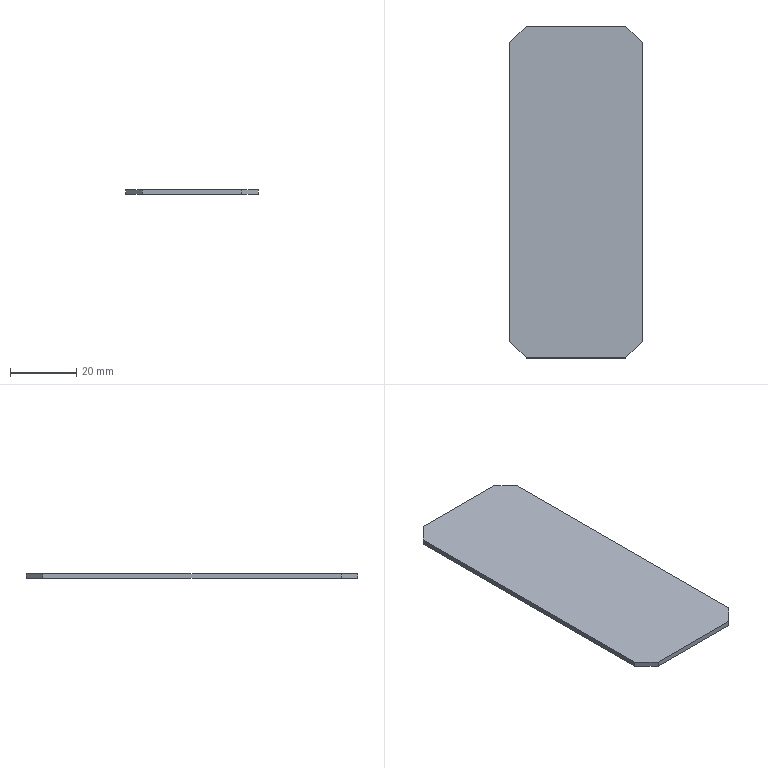Part | STEP file | Box reinforcing rib plate 001 | 1 solid | 10 faces | box 40 x 100 x 1.5 mm | volume 5925 mm3 | plane 10
STEP:
#1=CARTESIAN_POINT('',(0.,0.,0.));
#2=DIRECTION('',(0.,0.,1.));
#3=DIRECTION('',(1.,0.,0.));
#4=AXIS2_PLACEMENT_3D('',#1,#2,#3);
#5=CARTESIAN_POINT('',(20.,-45.,-0.75));
#6=VERTEX_POINT('',#5);
#7=CARTESIAN_POINT('',(20.,45.,-0.75));
#8=VERTEX_POINT('',#7);
#9=CARTESIAN_POINT('',(20.,-50.,-0.75));
#10=DIRECTION('',(0.,1.,0.));
#11=VECTOR('',#10,1.);
#12=LINE('',#9,#11);
#13=CARTESIAN_POINT('',(20.,-50.,0.75));
#14=DIRECTION('',(-1.,0.,0.));
#15=DIRECTION('',(0.,0.,1.));
#16=AXIS2_PLACEMENT_3D('',#13,#14,#15);
#17=PLANE('',#16);
#18=CARTESIAN_POINT('',(-1.5,0.));
#19=DIRECTION('',(0.,1.));
#20=VECTOR('',#19,1.);
#21=LINE('',#18,#20);
#22=(GEOMETRIC_REPRESENTATION_CONTEXT(2)PARAMETRIC_REPRESENTATION_CONTEXT()REPRESENTATION_CONTEXT('',''));
#23=DEFINITIONAL_REPRESENTATION('',(#21),#22);
#24=PCURVE('',#17,#23);
#25=CARTESIAN_POINT('',(0.,0.,-0.75));
#26=DIRECTION('',(0.,0.,-1.));
#27=DIRECTION('',(-1.,0.,0.));
#28=AXIS2_PLACEMENT_3D('',#25,#26,#27);
#29=PLANE('',#28);
#30=CARTESIAN_POINT('',(-20.,-50.));
#31=DIRECTION('',(0.,1.));
#32=VECTOR('',#31,1.);
#33=LINE('',#30,#32);
#34=(GEOMETRIC_REPRESENTATION_CONTEXT(2)PARAMETRIC_REPRESENTATION_CONTEXT()REPRESENTATION_CONTEXT('',''));
#35=DEFINITIONAL_REPRESENTATION('',(#33),#34);
#36=PCURVE('',#29,#35);
#37=SURFACE_CURVE('',#12,(#24,#36),.PCURVE_S1.);
#38=EDGE_CURVE('',#6,#8,#37,.T.);
#39=ORIENTED_EDGE('',*,*,#38,.T.);
#40=CARTESIAN_POINT('',(20.,45.,0.75));
#41=VERTEX_POINT('',#40);
#42=CARTESIAN_POINT('',(20.,45.,0.75));
#43=DIRECTION('',(0.,0.,1.));
#44=VECTOR('',#43,1.);
#45=LINE('',#42,#44);
#46=CARTESIAN_POINT('',(0.,95.));
#47=DIRECTION('',(1.,0.));
#48=VECTOR('',#47,1.);
#49=LINE('',#46,#48);
#50=(GEOMETRIC_REPRESENTATION_CONTEXT(2)PARAMETRIC_REPRESENTATION_CONTEXT()REPRESENTATION_CONTEXT('',''));
#51=DEFINITIONAL_REPRESENTATION('',(#49),#50);
#52=PCURVE('',#17,#51);
#53=CARTESIAN_POINT('',(15.,50.,0.75));
#54=DIRECTION('',(-0.7071,-0.7071,0.));
#55=DIRECTION('',(0.,0.,-1.));
#56=AXIS2_PLACEMENT_3D('',#53,#54,#55);
#57=PLANE('',#56);
#58=CARTESIAN_POINT('',(0.,7.071));
#59=DIRECTION('',(-1.,0.));
#60=VECTOR('',#59,1.);
#61=LINE('',#58,#60);
#62=(GEOMETRIC_REPRESENTATION_CONTEXT(2)PARAMETRIC_REPRESENTATION_CONTEXT()REPRESENTATION_CONTEXT('',''));
#63=DEFINITIONAL_REPRESENTATION('',(#61),#62);
#64=PCURVE('',#57,#63);
#65=SURFACE_CURVE('',#45,(#52,#64),.PCURVE_S1.);
#66=EDGE_CURVE('',#8,#41,#65,.T.);
#67=ORIENTED_EDGE('',*,*,#66,.T.);
#68=CARTESIAN_POINT('',(20.,-45.,0.75));
#69=VERTEX_POINT('',#68);
#70=CARTESIAN_POINT('',(20.,-50.,0.75));
#71=DIRECTION('',(0.,1.,0.));
#72=VECTOR('',#71,1.);
#73=LINE('',#70,#72);
#74=CARTESIAN_POINT('',(0.,0.));
#75=DIRECTION('',(0.,1.));
#76=VECTOR('',#75,1.);
#77=LINE('',#74,#76);
#78=(GEOMETRIC_REPRESENTATION_CONTEXT(2)PARAMETRIC_REPRESENTATION_CONTEXT()REPRESENTATION_CONTEXT('',''));
#79=DEFINITIONAL_REPRESENTATION('',(#77),#78);
#80=PCURVE('',#17,#79);
#81=CARTESIAN_POINT('',(0.,0.,0.75));
#82=DIRECTION('',(0.,0.,-1.));
#83=DIRECTION('',(-1.,0.,0.));
#84=AXIS2_PLACEMENT_3D('',#81,#82,#83);
#85=PLANE('',#84);
#86=CARTESIAN_POINT('',(-20.,-50.));
#87=DIRECTION('',(0.,1.));
#88=VECTOR('',#87,1.);
#89=LINE('',#86,#88);
#90=(GEOMETRIC_REPRESENTATION_CONTEXT(2)PARAMETRIC_REPRESENTATION_CONTEXT()REPRESENTATION_CONTEXT('',''));
#91=DEFINITIONAL_REPRESENTATION('',(#89),#90);
#92=PCURVE('',#85,#91);
#93=SURFACE_CURVE('',#73,(#80,#92),.PCURVE_S1.);
#94=EDGE_CURVE('',#69,#41,#93,.T.);
#95=ORIENTED_EDGE('',*,*,#94,.F.);
#96=CARTESIAN_POINT('',(20.,-45.,0.75));
#97=DIRECTION('',(0.,0.,-1.));
#98=VECTOR('',#97,1.);
#99=LINE('',#96,#98);
#100=CARTESIAN_POINT('',(0.,5.));
#101=DIRECTION('',(-1.,0.));
#102=VECTOR('',#101,1.);
#103=LINE('',#100,#102);
#104=(GEOMETRIC_REPRESENTATION_CONTEXT(2)PARAMETRIC_REPRESENTATION_CONTEXT()REPRESENTATION_CONTEXT('',''));
#105=DEFINITIONAL_REPRESENTATION('',(#103),#104);
#106=PCURVE('',#17,#105);
#107=CARTESIAN_POINT('',(20.,-45.,0.75));
#108=DIRECTION('',(-0.7071,0.7071,0.));
#109=DIRECTION('',(0.,0.,-1.));
#110=AXIS2_PLACEMENT_3D('',#107,#108,#109);
#111=PLANE('',#110);
#112=CARTESIAN_POINT('',(0.,0.));
#113=DIRECTION('',(1.,0.));
#114=VECTOR('',#113,1.);
#115=LINE('',#112,#114);
#116=(GEOMETRIC_REPRESENTATION_CONTEXT(2)PARAMETRIC_REPRESENTATION_CONTEXT()REPRESENTATION_CONTEXT('',''));
#117=DEFINITIONAL_REPRESENTATION('',(#115),#116);
#118=PCURVE('',#111,#117);
#119=SURFACE_CURVE('',#99,(#106,#118),.PCURVE_S1.);
#120=EDGE_CURVE('',#69,#6,#119,.T.);
#121=ORIENTED_EDGE('',*,*,#120,.T.);
#122=EDGE_LOOP('',(#39,#67,#95,#121));
#123=FACE_BOUND('',#122,.T.);
#124=ADVANCED_FACE('',(#123),#17,.F.);
#125=CARTESIAN_POINT('',(15.,50.,0.75));
#126=VERTEX_POINT('',#125);
#127=CARTESIAN_POINT('',(-15.,50.,0.75));
#128=VERTEX_POINT('',#127);
#129=CARTESIAN_POINT('',(-20.,50.,0.75));
#130=DIRECTION('',(-1.,0.,0.));
#131=VECTOR('',#130,1.);
#132=LINE('',#129,#131);
#133=CARTESIAN_POINT('',(-20.,50.,0.75));
#134=DIRECTION('',(0.,-1.,0.));
#135=DIRECTION('',(0.,0.,-1.));
#136=AXIS2_PLACEMENT_3D('',#133,#134,#135);
#137=PLANE('',#136);
#138=CARTESIAN_POINT('',(0.,0.));
#139=DIRECTION('',(0.,-1.));
#140=VECTOR('',#139,1.);
#141=LINE('',#138,#140);
#142=(GEOMETRIC_REPRESENTATION_CONTEXT(2)PARAMETRIC_REPRESENTATION_CONTEXT()REPRESENTATION_CONTEXT('',''));
#143=DEFINITIONAL_REPRESENTATION('',(#141),#142);
#144=PCURVE('',#137,#143);
#145=CARTESIAN_POINT('',(20.,50.));
#146=DIRECTION('',(1.,0.));
#147=VECTOR('',#146,1.);
#148=LINE('',#145,#147);
#149=(GEOMETRIC_REPRESENTATION_CONTEXT(2)PARAMETRIC_REPRESENTATION_CONTEXT()REPRESENTATION_CONTEXT('',''));
#150=DEFINITIONAL_REPRESENTATION('',(#148),#149);
#151=PCURVE('',#85,#150);
#152=SURFACE_CURVE('',#132,(#144,#151),.PCURVE_S1.);
#153=EDGE_CURVE('',#126,#128,#152,.T.);
#154=ORIENTED_EDGE('',*,*,#153,.F.);
#155=CARTESIAN_POINT('',(15.,50.,-0.75));
#156=VERTEX_POINT('',#155);
#157=CARTESIAN_POINT('',(15.,50.,0.75));
#158=DIRECTION('',(0.,0.,-1.));
#159=VECTOR('',#158,1.);
#160=LINE('',#157,#159);
#161=CARTESIAN_POINT('',(0.,35.));
#162=DIRECTION('',(1.,0.));
#163=VECTOR('',#162,1.);
#164=LINE('',#161,#163);
#165=(GEOMETRIC_REPRESENTATION_CONTEXT(2)PARAMETRIC_REPRESENTATION_CONTEXT()REPRESENTATION_CONTEXT('',''));
#166=DEFINITIONAL_REPRESENTATION('',(#164),#165);
#167=PCURVE('',#137,#166);
#168=CARTESIAN_POINT('',(0.,0.));
#169=DIRECTION('',(1.,0.));
#170=VECTOR('',#169,1.);
#171=LINE('',#168,#170);
#172=(GEOMETRIC_REPRESENTATION_CONTEXT(2)PARAMETRIC_REPRESENTATION_CONTEXT()REPRESENTATION_CONTEXT('',''));
#173=DEFINITIONAL_REPRESENTATION('',(#171),#172);
#174=PCURVE('',#57,#173);
#175=SURFACE_CURVE('',#160,(#167,#174),.PCURVE_S1.);
#176=EDGE_CURVE('',#126,#156,#175,.T.);
#177=ORIENTED_EDGE('',*,*,#176,.T.);
#178=CARTESIAN_POINT('',(-15.,50.,-0.75));
#179=VERTEX_POINT('',#178);
#180=CARTESIAN_POINT('',(-20.,50.,-0.75));
#181=DIRECTION('',(-1.,0.,0.));
#182=VECTOR('',#181,1.);
#183=LINE('',#180,#182);
#184=CARTESIAN_POINT('',(1.5,0.));
#185=DIRECTION('',(0.,-1.));
#186=VECTOR('',#185,1.);
#187=LINE('',#184,#186);
#188=(GEOMETRIC_REPRESENTATION_CONTEXT(2)PARAMETRIC_REPRESENTATION_CONTEXT()REPRESENTATION_CONTEXT('',''));
#189=DEFINITIONAL_REPRESENTATION('',(#187),#188);
#190=PCURVE('',#137,#189);
#191=CARTESIAN_POINT('',(20.,50.));
#192=DIRECTION('',(1.,0.));
#193=VECTOR('',#192,1.);
#194=LINE('',#191,#193);
#195=(GEOMETRIC_REPRESENTATION_CONTEXT(2)PARAMETRIC_REPRESENTATION_CONTEXT()REPRESENTATION_CONTEXT('',''));
#196=DEFINITIONAL_REPRESENTATION('',(#194),#195);
#197=PCURVE('',#29,#196);
#198=SURFACE_CURVE('',#183,(#190,#197),.PCURVE_S1.);
#199=EDGE_CURVE('',#156,#179,#198,.T.);
#200=ORIENTED_EDGE('',*,*,#199,.T.);
#201=CARTESIAN_POINT('',(-15.,50.,0.75));
#202=DIRECTION('',(0.,0.,1.));
#203=VECTOR('',#202,1.);
#204=LINE('',#201,#203);
#205=CARTESIAN_POINT('',(0.,5.));
#206=DIRECTION('',(-1.,0.));
#207=VECTOR('',#206,1.);
#208=LINE('',#205,#207);
#209=(GEOMETRIC_REPRESENTATION_CONTEXT(2)PARAMETRIC_REPRESENTATION_CONTEXT()REPRESENTATION_CONTEXT('',''));
#210=DEFINITIONAL_REPRESENTATION('',(#208),#209);
#211=PCURVE('',#137,#210);
#212=CARTESIAN_POINT('',(-20.,45.,0.75));
#213=DIRECTION('',(0.7071,-0.7071,0.));
#214=DIRECTION('',(0.,0.,-1.));
#215=AXIS2_PLACEMENT_3D('',#212,#213,#214);
#216=PLANE('',#215);
#217=CARTESIAN_POINT('',(0.,7.071));
#218=DIRECTION('',(-1.,0.));
#219=VECTOR('',#218,1.);
#220=LINE('',#217,#219);
#221=(GEOMETRIC_REPRESENTATION_CONTEXT(2)PARAMETRIC_REPRESENTATION_CONTEXT()REPRESENTATION_CONTEXT('',''));
#222=DEFINITIONAL_REPRESENTATION('',(#220),#221);
#223=PCURVE('',#216,#222);
#224=SURFACE_CURVE('',#204,(#211,#223),.PCURVE_S1.);
#225=EDGE_CURVE('',#179,#128,#224,.T.);
#226=ORIENTED_EDGE('',*,*,#225,.T.);
#227=EDGE_LOOP('',(#154,#177,#200,#226));
#228=FACE_BOUND('',#227,.T.);
#229=ADVANCED_FACE('',(#228),#137,.F.);
#230=CARTESIAN_POINT('',(-20.,45.,-0.75));
#231=VERTEX_POINT('',#230);
#232=CARTESIAN_POINT('',(-20.,-45.,-0.75));
#233=VERTEX_POINT('',#232);
#234=CARTESIAN_POINT('',(-20.,-50.,-0.75));
#235=DIRECTION('',(0.,-1.,0.));
#236=VECTOR('',#235,1.);
#237=LINE('',#234,#236);
#238=CARTESIAN_POINT('',(-20.,-50.,0.75));
#239=DIRECTION('',(1.,0.,0.));
#240=DIRECTION('',(0.,0.,-1.));
#241=AXIS2_PLACEMENT_3D('',#238,#239,#240);
#242=PLANE('',#241);
#243=CARTESIAN_POINT('',(1.5,0.));
#244=DIRECTION('',(0.,-1.));
#245=VECTOR('',#244,1.);
#246=LINE('',#243,#245);
#247=(GEOMETRIC_REPRESENTATION_CONTEXT(2)PARAMETRIC_REPRESENTATION_CONTEXT()REPRESENTATION_CONTEXT('',''));
#248=DEFINITIONAL_REPRESENTATION('',(#246),#247);
#249=PCURVE('',#242,#248);
#250=CARTESIAN_POINT('',(20.,-50.));
#251=DIRECTION('',(0.,-1.));
#252=VECTOR('',#251,1.);
#253=LINE('',#250,#252);
#254=(GEOMETRIC_REPRESENTATION_CONTEXT(2)PARAMETRIC_REPRESENTATION_CONTEXT()REPRESENTATION_CONTEXT('',''));
#255=DEFINITIONAL_REPRESENTATION('',(#253),#254);
#256=PCURVE('',#29,#255);
#257=SURFACE_CURVE('',#237,(#249,#256),.PCURVE_S1.);
#258=EDGE_CURVE('',#231,#233,#257,.T.);
#259=ORIENTED_EDGE('',*,*,#258,.T.);
#260=CARTESIAN_POINT('',(-20.,-45.,0.75));
#261=VERTEX_POINT('',#260);
#262=CARTESIAN_POINT('',(-20.,-45.,0.75));
#263=DIRECTION('',(0.,0.,1.));
#264=VECTOR('',#263,1.);
#265=LINE('',#262,#264);
#266=CARTESIAN_POINT('',(0.,5.));
#267=DIRECTION('',(-1.,0.));
#268=VECTOR('',#267,1.);
#269=LINE('',#266,#268);
#270=(GEOMETRIC_REPRESENTATION_CONTEXT(2)PARAMETRIC_REPRESENTATION_CONTEXT()REPRESENTATION_CONTEXT('',''));
#271=DEFINITIONAL_REPRESENTATION('',(#269),#270);
#272=PCURVE('',#242,#271);
#273=CARTESIAN_POINT('',(-15.,-50.,0.75));
#274=DIRECTION('',(0.7071,0.7071,0.));
#275=DIRECTION('',(0.,0.,-1.));
#276=AXIS2_PLACEMENT_3D('',#273,#274,#275);
#277=PLANE('',#276);
#278=CARTESIAN_POINT('',(0.,7.071));
#279=DIRECTION('',(-1.,0.));
#280=VECTOR('',#279,1.);
#281=LINE('',#278,#280);
#282=(GEOMETRIC_REPRESENTATION_CONTEXT(2)PARAMETRIC_REPRESENTATION_CONTEXT()REPRESENTATION_CONTEXT('',''));
#283=DEFINITIONAL_REPRESENTATION('',(#281),#282);
#284=PCURVE('',#277,#283);
#285=SURFACE_CURVE('',#265,(#272,#284),.PCURVE_S1.);
#286=EDGE_CURVE('',#233,#261,#285,.T.);
#287=ORIENTED_EDGE('',*,*,#286,.T.);
#288=CARTESIAN_POINT('',(-20.,45.,0.75));
#289=VERTEX_POINT('',#288);
#290=CARTESIAN_POINT('',(-20.,-50.,0.75));
#291=DIRECTION('',(0.,-1.,0.));
#292=VECTOR('',#291,1.);
#293=LINE('',#290,#292);
#294=CARTESIAN_POINT('',(0.,0.));
#295=DIRECTION('',(0.,-1.));
#296=VECTOR('',#295,1.);
#297=LINE('',#294,#296);
#298=(GEOMETRIC_REPRESENTATION_CONTEXT(2)PARAMETRIC_REPRESENTATION_CONTEXT()REPRESENTATION_CONTEXT('',''));
#299=DEFINITIONAL_REPRESENTATION('',(#297),#298);
#300=PCURVE('',#242,#299);
#301=CARTESIAN_POINT('',(20.,-50.));
#302=DIRECTION('',(0.,-1.));
#303=VECTOR('',#302,1.);
#304=LINE('',#301,#303);
#305=(GEOMETRIC_REPRESENTATION_CONTEXT(2)PARAMETRIC_REPRESENTATION_CONTEXT()REPRESENTATION_CONTEXT('',''));
#306=DEFINITIONAL_REPRESENTATION('',(#304),#305);
#307=PCURVE('',#85,#306);
#308=SURFACE_CURVE('',#293,(#300,#307),.PCURVE_S1.);
#309=EDGE_CURVE('',#289,#261,#308,.T.);
#310=ORIENTED_EDGE('',*,*,#309,.F.);
#311=CARTESIAN_POINT('',(-20.,45.,0.75));
#312=DIRECTION('',(0.,0.,-1.));
#313=VECTOR('',#312,1.);
#314=LINE('',#311,#313);
#315=CARTESIAN_POINT('',(0.,95.));
#316=DIRECTION('',(1.,0.));
#317=VECTOR('',#316,1.);
#318=LINE('',#315,#317);
#319=(GEOMETRIC_REPRESENTATION_CONTEXT(2)PARAMETRIC_REPRESENTATION_CONTEXT()REPRESENTATION_CONTEXT('',''));
#320=DEFINITIONAL_REPRESENTATION('',(#318),#319);
#321=PCURVE('',#242,#320);
#322=CARTESIAN_POINT('',(0.,0.));
#323=DIRECTION('',(1.,0.));
#324=VECTOR('',#323,1.);
#325=LINE('',#322,#324);
#326=(GEOMETRIC_REPRESENTATION_CONTEXT(2)PARAMETRIC_REPRESENTATION_CONTEXT()REPRESENTATION_CONTEXT('',''));
#327=DEFINITIONAL_REPRESENTATION('',(#325),#326);
#328=PCURVE('',#216,#327);
#329=SURFACE_CURVE('',#314,(#321,#328),.PCURVE_S1.);
#330=EDGE_CURVE('',#289,#231,#329,.T.);
#331=ORIENTED_EDGE('',*,*,#330,.T.);
#332=EDGE_LOOP('',(#259,#287,#310,#331));
#333=FACE_BOUND('',#332,.T.);
#334=ADVANCED_FACE('',(#333),#242,.F.);
#335=CARTESIAN_POINT('',(-15.,-50.,0.75));
#336=VERTEX_POINT('',#335);
#337=CARTESIAN_POINT('',(15.,-50.,0.75));
#338=VERTEX_POINT('',#337);
#339=CARTESIAN_POINT('',(-20.,-50.,0.75));
#340=DIRECTION('',(1.,0.,0.));
#341=VECTOR('',#340,1.);
#342=LINE('',#339,#341);
#343=CARTESIAN_POINT('',(-20.,-50.,0.75));
#344=DIRECTION('',(0.,1.,0.));
#345=DIRECTION('',(0.,0.,1.));
#346=AXIS2_PLACEMENT_3D('',#343,#344,#345);
#347=PLANE('',#346);
#348=CARTESIAN_POINT('',(0.,0.));
#349=DIRECTION('',(0.,1.));
#350=VECTOR('',#349,1.);
#351=LINE('',#348,#350);
#352=(GEOMETRIC_REPRESENTATION_CONTEXT(2)PARAMETRIC_REPRESENTATION_CONTEXT()REPRESENTATION_CONTEXT('',''));
#353=DEFINITIONAL_REPRESENTATION('',(#351),#352);
#354=PCURVE('',#347,#353);
#355=CARTESIAN_POINT('',(20.,-50.));
#356=DIRECTION('',(-1.,0.));
#357=VECTOR('',#356,1.);
#358=LINE('',#355,#357);
#359=(GEOMETRIC_REPRESENTATION_CONTEXT(2)PARAMETRIC_REPRESENTATION_CONTEXT()REPRESENTATION_CONTEXT('',''));
#360=DEFINITIONAL_REPRESENTATION('',(#358),#359);
#361=PCURVE('',#85,#360);
#362=SURFACE_CURVE('',#342,(#354,#361),.PCURVE_S1.);
#363=EDGE_CURVE('',#336,#338,#362,.T.);
#364=ORIENTED_EDGE('',*,*,#363,.F.);
#365=CARTESIAN_POINT('',(-15.,-50.,-0.75));
#366=VERTEX_POINT('',#365);
#367=CARTESIAN_POINT('',(-15.,-50.,0.75));
#368=DIRECTION('',(0.,0.,-1.));
#369=VECTOR('',#368,1.);
#370=LINE('',#367,#369);
#371=CARTESIAN_POINT('',(0.,5.));
#372=DIRECTION('',(-1.,0.));
#373=VECTOR('',#372,1.);
#374=LINE('',#371,#373);
#375=(GEOMETRIC_REPRESENTATION_CONTEXT(2)PARAMETRIC_REPRESENTATION_CONTEXT()REPRESENTATION_CONTEXT('',''));
#376=DEFINITIONAL_REPRESENTATION('',(#374),#375);
#377=PCURVE('',#347,#376);
#378=CARTESIAN_POINT('',(0.,0.));
#379=DIRECTION('',(1.,0.));
#380=VECTOR('',#379,1.);
#381=LINE('',#378,#380);
#382=(GEOMETRIC_REPRESENTATION_CONTEXT(2)PARAMETRIC_REPRESENTATION_CONTEXT()REPRESENTATION_CONTEXT('',''));
#383=DEFINITIONAL_REPRESENTATION('',(#381),#382);
#384=PCURVE('',#277,#383);
#385=SURFACE_CURVE('',#370,(#377,#384),.PCURVE_S1.);
#386=EDGE_CURVE('',#336,#366,#385,.T.);
#387=ORIENTED_EDGE('',*,*,#386,.T.);
#388=CARTESIAN_POINT('',(15.,-50.,-0.75));
#389=VERTEX_POINT('',#388);
#390=CARTESIAN_POINT('',(-20.,-50.,-0.75));
#391=DIRECTION('',(1.,0.,0.));
#392=VECTOR('',#391,1.);
#393=LINE('',#390,#392);
#394=CARTESIAN_POINT('',(-1.5,0.));
#395=DIRECTION('',(0.,1.));
#396=VECTOR('',#395,1.);
#397=LINE('',#394,#396);
#398=(GEOMETRIC_REPRESENTATION_CONTEXT(2)PARAMETRIC_REPRESENTATION_CONTEXT()REPRESENTATION_CONTEXT('',''));
#399=DEFINITIONAL_REPRESENTATION('',(#397),#398);
#400=PCURVE('',#347,#399);
#401=CARTESIAN_POINT('',(20.,-50.));
#402=DIRECTION('',(-1.,0.));
#403=VECTOR('',#402,1.);
#404=LINE('',#401,#403);
#405=(GEOMETRIC_REPRESENTATION_CONTEXT(2)PARAMETRIC_REPRESENTATION_CONTEXT()REPRESENTATION_CONTEXT('',''));
#406=DEFINITIONAL_REPRESENTATION('',(#404),#405);
#407=PCURVE('',#29,#406);
#408=SURFACE_CURVE('',#393,(#400,#407),.PCURVE_S1.);
#409=EDGE_CURVE('',#366,#389,#408,.T.);
#410=ORIENTED_EDGE('',*,*,#409,.T.);
#411=CARTESIAN_POINT('',(15.,-50.,0.75));
#412=DIRECTION('',(0.,0.,1.));
#413=VECTOR('',#412,1.);
#414=LINE('',#411,#413);
#415=CARTESIAN_POINT('',(0.,35.));
#416=DIRECTION('',(1.,0.));
#417=VECTOR('',#416,1.);
#418=LINE('',#415,#417);
#419=(GEOMETRIC_REPRESENTATION_CONTEXT(2)PARAMETRIC_REPRESENTATION_CONTEXT()REPRESENTATION_CONTEXT('',''));
#420=DEFINITIONAL_REPRESENTATION('',(#418),#419);
#421=PCURVE('',#347,#420);
#422=CARTESIAN_POINT('',(0.,7.071));
#423=DIRECTION('',(-1.,0.));
#424=VECTOR('',#423,1.);
#425=LINE('',#422,#424);
#426=(GEOMETRIC_REPRESENTATION_CONTEXT(2)PARAMETRIC_REPRESENTATION_CONTEXT()REPRESENTATION_CONTEXT('',''));
#427=DEFINITIONAL_REPRESENTATION('',(#425),#426);
#428=PCURVE('',#111,#427);
#429=SURFACE_CURVE('',#414,(#421,#428),.PCURVE_S1.);
#430=EDGE_CURVE('',#389,#338,#429,.T.);
#431=ORIENTED_EDGE('',*,*,#430,.T.);
#432=EDGE_LOOP('',(#364,#387,#410,#431));
#433=FACE_BOUND('',#432,.T.);
#434=ADVANCED_FACE('',(#433),#347,.F.);
#435=ORIENTED_EDGE('',*,*,#94,.T.);
#436=CARTESIAN_POINT('',(15.,50.,0.75));
#437=DIRECTION('',(-0.7071,0.7071,0.));
#438=VECTOR('',#437,1.);
#439=LINE('',#436,#438);
#440=CARTESIAN_POINT('',(-15.,50.));
#441=DIRECTION('',(0.7071,0.7071));
#442=VECTOR('',#441,1.);
#443=LINE('',#440,#442);
#444=(GEOMETRIC_REPRESENTATION_CONTEXT(2)PARAMETRIC_REPRESENTATION_CONTEXT()REPRESENTATION_CONTEXT('',''));
#445=DEFINITIONAL_REPRESENTATION('',(#443),#444);
#446=PCURVE('',#85,#445);
#447=CARTESIAN_POINT('',(0.,0.));
#448=DIRECTION('',(0.,-1.));
#449=VECTOR('',#448,1.);
#450=LINE('',#447,#449);
#451=(GEOMETRIC_REPRESENTATION_CONTEXT(2)PARAMETRIC_REPRESENTATION_CONTEXT()REPRESENTATION_CONTEXT('',''));
#452=DEFINITIONAL_REPRESENTATION('',(#450),#451);
#453=PCURVE('',#57,#452);
#454=SURFACE_CURVE('',#439,(#446,#453),.PCURVE_S1.);
#455=EDGE_CURVE('',#41,#126,#454,.T.);
#456=ORIENTED_EDGE('',*,*,#455,.T.);
#457=ORIENTED_EDGE('',*,*,#153,.T.);
#458=CARTESIAN_POINT('',(-20.,45.,0.75));
#459=DIRECTION('',(-0.7071,-0.7071,0.));
#460=VECTOR('',#459,1.);
#461=LINE('',#458,#460);
#462=CARTESIAN_POINT('',(20.,45.));
#463=DIRECTION('',(0.7071,-0.7071));
#464=VECTOR('',#463,1.);
#465=LINE('',#462,#464);
#466=(GEOMETRIC_REPRESENTATION_CONTEXT(2)PARAMETRIC_REPRESENTATION_CONTEXT()REPRESENTATION_CONTEXT('',''));
#467=DEFINITIONAL_REPRESENTATION('',(#465),#466);
#468=PCURVE('',#85,#467);
#469=CARTESIAN_POINT('',(0.,0.));
#470=DIRECTION('',(0.,-1.));
#471=VECTOR('',#470,1.);
#472=LINE('',#469,#471);
#473=(GEOMETRIC_REPRESENTATION_CONTEXT(2)PARAMETRIC_REPRESENTATION_CONTEXT()REPRESENTATION_CONTEXT('',''));
#474=DEFINITIONAL_REPRESENTATION('',(#472),#473);
#475=PCURVE('',#216,#474);
#476=SURFACE_CURVE('',#461,(#468,#475),.PCURVE_S1.);
#477=EDGE_CURVE('',#128,#289,#476,.T.);
#478=ORIENTED_EDGE('',*,*,#477,.T.);
#479=ORIENTED_EDGE('',*,*,#309,.T.);
#480=CARTESIAN_POINT('',(-15.,-50.,0.75));
#481=DIRECTION('',(0.7071,-0.7071,0.));
#482=VECTOR('',#481,1.);
#483=LINE('',#480,#482);
#484=CARTESIAN_POINT('',(15.,-50.));
#485=DIRECTION('',(-0.7071,-0.7071));
#486=VECTOR('',#485,1.);
#487=LINE('',#484,#486);
#488=(GEOMETRIC_REPRESENTATION_CONTEXT(2)PARAMETRIC_REPRESENTATION_CONTEXT()REPRESENTATION_CONTEXT('',''));
#489=DEFINITIONAL_REPRESENTATION('',(#487),#488);
#490=PCURVE('',#85,#489);
#491=CARTESIAN_POINT('',(0.,0.));
#492=DIRECTION('',(0.,-1.));
#493=VECTOR('',#492,1.);
#494=LINE('',#491,#493);
#495=(GEOMETRIC_REPRESENTATION_CONTEXT(2)PARAMETRIC_REPRESENTATION_CONTEXT()REPRESENTATION_CONTEXT('',''));
#496=DEFINITIONAL_REPRESENTATION('',(#494),#495);
#497=PCURVE('',#277,#496);
#498=SURFACE_CURVE('',#483,(#490,#497),.PCURVE_S1.);
#499=EDGE_CURVE('',#261,#336,#498,.T.);
#500=ORIENTED_EDGE('',*,*,#499,.T.);
#501=ORIENTED_EDGE('',*,*,#363,.T.);
#502=CARTESIAN_POINT('',(20.,-45.,0.75));
#503=DIRECTION('',(0.7071,0.7071,0.));
#504=VECTOR('',#503,1.);
#505=LINE('',#502,#504);
#506=CARTESIAN_POINT('',(-20.,-45.));
#507=DIRECTION('',(-0.7071,0.7071));
#508=VECTOR('',#507,1.);
#509=LINE('',#506,#508);
#510=(GEOMETRIC_REPRESENTATION_CONTEXT(2)PARAMETRIC_REPRESENTATION_CONTEXT()REPRESENTATION_CONTEXT('',''));
#511=DEFINITIONAL_REPRESENTATION('',(#509),#510);
#512=PCURVE('',#85,#511);
#513=CARTESIAN_POINT('',(0.,0.));
#514=DIRECTION('',(0.,-1.));
#515=VECTOR('',#514,1.);
#516=LINE('',#513,#515);
#517=(GEOMETRIC_REPRESENTATION_CONTEXT(2)PARAMETRIC_REPRESENTATION_CONTEXT()REPRESENTATION_CONTEXT('',''));
#518=DEFINITIONAL_REPRESENTATION('',(#516),#517);
#519=PCURVE('',#111,#518);
#520=SURFACE_CURVE('',#505,(#512,#519),.PCURVE_S1.);
#521=EDGE_CURVE('',#338,#69,#520,.T.);
#522=ORIENTED_EDGE('',*,*,#521,.T.);
#523=EDGE_LOOP('',(#435,#456,#457,#478,#479,#500,#501,#522));
#524=FACE_BOUND('',#523,.T.);
#525=ADVANCED_FACE('',(#524),#85,.F.);
#526=ORIENTED_EDGE('',*,*,#199,.F.);
#527=CARTESIAN_POINT('',(32.5,32.5,-0.75));
#528=DIRECTION('',(0.7071,-0.7071,0.));
#529=VECTOR('',#528,1.);
#530=LINE('',#527,#529);
#531=CARTESIAN_POINT('',(-32.5,32.5));
#532=DIRECTION('',(-0.7071,-0.7071));
#533=VECTOR('',#532,1.);
#534=LINE('',#531,#533);
#535=(GEOMETRIC_REPRESENTATION_CONTEXT(2)PARAMETRIC_REPRESENTATION_CONTEXT()REPRESENTATION_CONTEXT('',''));
#536=DEFINITIONAL_REPRESENTATION('',(#534),#535);
#537=PCURVE('',#29,#536);
#538=CARTESIAN_POINT('',(1.5,24.749));
#539=DIRECTION('',(0.,1.));
#540=VECTOR('',#539,1.);
#541=LINE('',#538,#540);
#542=(GEOMETRIC_REPRESENTATION_CONTEXT(2)PARAMETRIC_REPRESENTATION_CONTEXT()REPRESENTATION_CONTEXT('',''));
#543=DEFINITIONAL_REPRESENTATION('',(#541),#542);
#544=PCURVE('',#57,#543);
#545=SURFACE_CURVE('',#530,(#537,#544),.PCURVE_S1.);
#546=EDGE_CURVE('',#156,#8,#545,.T.);
#547=ORIENTED_EDGE('',*,*,#546,.T.);
#548=ORIENTED_EDGE('',*,*,#38,.F.);
#549=CARTESIAN_POINT('',(32.5,-32.5,-0.75));
#550=DIRECTION('',(-0.7071,-0.7071,0.));
#551=VECTOR('',#550,1.);
#552=LINE('',#549,#551);
#553=CARTESIAN_POINT('',(-32.5,-32.5));
#554=DIRECTION('',(0.7071,-0.7071));
#555=VECTOR('',#554,1.);
#556=LINE('',#553,#555);
#557=(GEOMETRIC_REPRESENTATION_CONTEXT(2)PARAMETRIC_REPRESENTATION_CONTEXT()REPRESENTATION_CONTEXT('',''));
#558=DEFINITIONAL_REPRESENTATION('',(#556),#557);
#559=PCURVE('',#29,#558);
#560=CARTESIAN_POINT('',(1.5,-17.678));
#561=DIRECTION('',(0.,1.));
#562=VECTOR('',#561,1.);
#563=LINE('',#560,#562);
#564=(GEOMETRIC_REPRESENTATION_CONTEXT(2)PARAMETRIC_REPRESENTATION_CONTEXT()REPRESENTATION_CONTEXT('',''));
#565=DEFINITIONAL_REPRESENTATION('',(#563),#564);
#566=PCURVE('',#111,#565);
#567=SURFACE_CURVE('',#552,(#559,#566),.PCURVE_S1.);
#568=EDGE_CURVE('',#6,#389,#567,.T.);
#569=ORIENTED_EDGE('',*,*,#568,.T.);
#570=ORIENTED_EDGE('',*,*,#409,.F.);
#571=CARTESIAN_POINT('',(-32.5,-32.5,-0.75));
#572=DIRECTION('',(-0.7071,0.7071,0.));
#573=VECTOR('',#572,1.);
#574=LINE('',#571,#573);
#575=CARTESIAN_POINT('',(32.5,-32.5));
#576=DIRECTION('',(0.7071,0.7071));
#577=VECTOR('',#576,1.);
#578=LINE('',#575,#577);
#579=(GEOMETRIC_REPRESENTATION_CONTEXT(2)PARAMETRIC_REPRESENTATION_CONTEXT()REPRESENTATION_CONTEXT('',''));
#580=DEFINITIONAL_REPRESENTATION('',(#578),#579);
#581=PCURVE('',#29,#580);
#582=CARTESIAN_POINT('',(1.5,24.749));
#583=DIRECTION('',(0.,1.));
#584=VECTOR('',#583,1.);
#585=LINE('',#582,#584);
#586=(GEOMETRIC_REPRESENTATION_CONTEXT(2)PARAMETRIC_REPRESENTATION_CONTEXT()REPRESENTATION_CONTEXT('',''));
#587=DEFINITIONAL_REPRESENTATION('',(#585),#586);
#588=PCURVE('',#277,#587);
#589=SURFACE_CURVE('',#574,(#581,#588),.PCURVE_S1.);
#590=EDGE_CURVE('',#366,#233,#589,.T.);
#591=ORIENTED_EDGE('',*,*,#590,.T.);
#592=ORIENTED_EDGE('',*,*,#258,.F.);
#593=CARTESIAN_POINT('',(-32.5,32.5,-0.75));
#594=DIRECTION('',(0.7071,0.7071,0.));
#595=VECTOR('',#594,1.);
#596=LINE('',#593,#595);
#597=CARTESIAN_POINT('',(32.5,32.5));
#598=DIRECTION('',(-0.7071,0.7071));
#599=VECTOR('',#598,1.);
#600=LINE('',#597,#599);
#601=(GEOMETRIC_REPRESENTATION_CONTEXT(2)PARAMETRIC_REPRESENTATION_CONTEXT()REPRESENTATION_CONTEXT('',''));
#602=DEFINITIONAL_REPRESENTATION('',(#600),#601);
#603=PCURVE('',#29,#602);
#604=CARTESIAN_POINT('',(1.5,-17.678));
#605=DIRECTION('',(0.,1.));
#606=VECTOR('',#605,1.);
#607=LINE('',#604,#606);
#608=(GEOMETRIC_REPRESENTATION_CONTEXT(2)PARAMETRIC_REPRESENTATION_CONTEXT()REPRESENTATION_CONTEXT('',''));
#609=DEFINITIONAL_REPRESENTATION('',(#607),#608);
#610=PCURVE('',#216,#609);
#611=SURFACE_CURVE('',#596,(#603,#610),.PCURVE_S1.);
#612=EDGE_CURVE('',#231,#179,#611,.T.);
#613=ORIENTED_EDGE('',*,*,#612,.T.);
#614=EDGE_LOOP('',(#526,#547,#548,#569,#570,#591,#592,#613));
#615=FACE_BOUND('',#614,.T.);
#616=ADVANCED_FACE('',(#615),#29,.T.);
#617=ORIENTED_EDGE('',*,*,#455,.F.);
#618=ORIENTED_EDGE('',*,*,#66,.F.);
#619=ORIENTED_EDGE('',*,*,#546,.F.);
#620=ORIENTED_EDGE('',*,*,#176,.F.);
#621=EDGE_LOOP('',(#617,#618,#619,#620));
#622=FACE_BOUND('',#621,.T.);
#623=ADVANCED_FACE('',(#622),#57,.F.);
#624=ORIENTED_EDGE('',*,*,#499,.F.);
#625=ORIENTED_EDGE('',*,*,#286,.F.);
#626=ORIENTED_EDGE('',*,*,#590,.F.);
#627=ORIENTED_EDGE('',*,*,#386,.F.);
#628=EDGE_LOOP('',(#624,#625,#626,#627));
#629=FACE_BOUND('',#628,.T.);
#630=ADVANCED_FACE('',(#629),#277,.F.);
#631=ORIENTED_EDGE('',*,*,#477,.F.);
#632=ORIENTED_EDGE('',*,*,#225,.F.);
#633=ORIENTED_EDGE('',*,*,#612,.F.);
#634=ORIENTED_EDGE('',*,*,#330,.F.);
#635=EDGE_LOOP('',(#631,#632,#633,#634));
#636=FACE_BOUND('',#635,.T.);
#637=ADVANCED_FACE('',(#636),#216,.F.);
#638=ORIENTED_EDGE('',*,*,#521,.F.);
#639=ORIENTED_EDGE('',*,*,#430,.F.);
#640=ORIENTED_EDGE('',*,*,#568,.F.);
#641=ORIENTED_EDGE('',*,*,#120,.F.);
#642=EDGE_LOOP('',(#638,#639,#640,#641));
#643=FACE_BOUND('',#642,.T.);
#644=ADVANCED_FACE('',(#643),#111,.F.);
#645=CLOSED_SHELL('',(#124,#229,#334,#434,#525,#616,#623,#630,#637,#644));
#646=MANIFOLD_SOLID_BREP('',#645);
#647=(LENGTH_UNIT()NAMED_UNIT(*)SI_UNIT(.MILLI.,.METRE.));
#648=UNCERTAINTY_MEASURE_WITH_UNIT(LENGTH_MEASURE(0.0000001),#647,'','');
#649=(NAMED_UNIT(*)PLANE_ANGLE_UNIT()SI_UNIT($,.RADIAN.));
#650=(NAMED_UNIT(*)SI_UNIT($,.STERADIAN.)SOLID_ANGLE_UNIT());
#651=(GEOMETRIC_REPRESENTATION_CONTEXT(3)GLOBAL_UNCERTAINTY_ASSIGNED_CONTEXT((#648))GLOBAL_UNIT_ASSIGNED_CONTEXT((#647,#649,#650))REPRESENTATION_CONTEXT('',''));
#652=ADVANCED_BREP_SHAPE_REPRESENTATION('',(#4,#646),#651);